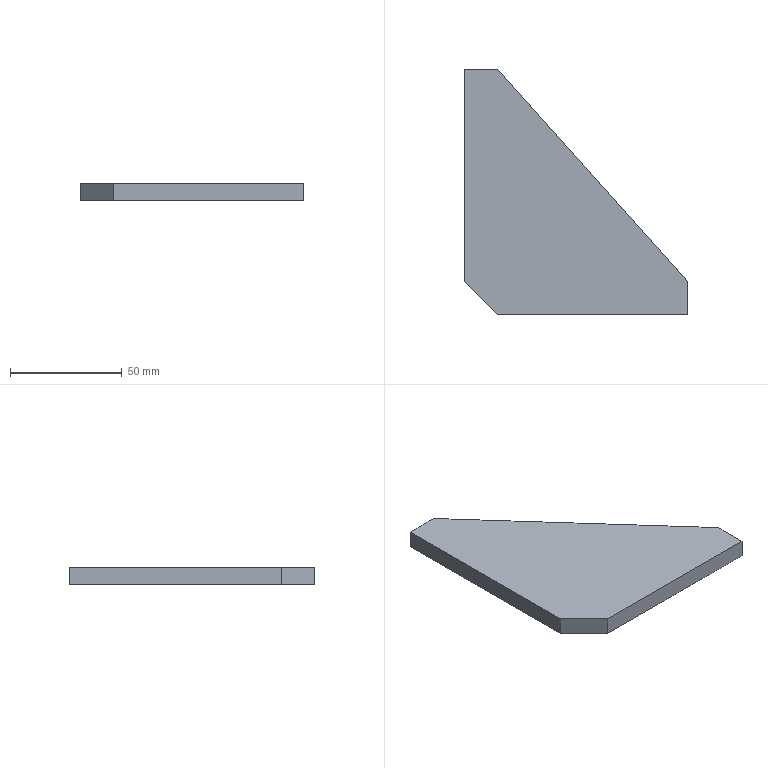Part | SolidWorks | features Chamfer 1, Extrusion 1 | 1 solid | 8 faces | box 100 x 110 x 8 mm | volume 54800 mm3 | plane 8
STEP:
#1=CARTESIAN_POINT('',(0.,110.,0.));
#2=VERTEX_POINT('',#1);
#3=CARTESIAN_POINT('',(0.,15.,0.));
#4=VERTEX_POINT('',#3);
#5=CARTESIAN_POINT('',(0.,110.,0.));
#6=DIRECTION('',(0.,-1.,0.));
#7=VECTOR('',#6,1000.);
#8=LINE('',#5,#7);
#9=EDGE_CURVE('',#2,#4,#8,.T.);
#10=ORIENTED_EDGE('',*,*,#9,.T.);
#11=CARTESIAN_POINT('',(0.,15.,8.));
#12=VERTEX_POINT('',#11);
#13=CARTESIAN_POINT('',(0.,15.,8.));
#14=DIRECTION('',(0.,0.,1.));
#15=VECTOR('',#14,1000.);
#16=LINE('',#13,#15);
#17=EDGE_CURVE('',#4,#12,#16,.T.);
#18=ORIENTED_EDGE('',*,*,#17,.T.);
#19=CARTESIAN_POINT('',(0.,110.,8.));
#20=VERTEX_POINT('',#19);
#21=CARTESIAN_POINT('',(0.,110.,8.));
#22=DIRECTION('',(0.,-1.,0.));
#23=VECTOR('',#22,1000.);
#24=LINE('',#21,#23);
#25=EDGE_CURVE('',#20,#12,#24,.T.);
#26=ORIENTED_EDGE('',*,*,#25,.F.);
#27=CARTESIAN_POINT('',(0.,110.,8.));
#28=DIRECTION('',(0.,0.,-1.));
#29=VECTOR('',#28,1000.);
#30=LINE('',#27,#29);
#31=EDGE_CURVE('',#20,#2,#30,.T.);
#32=ORIENTED_EDGE('',*,*,#31,.T.);
#33=EDGE_LOOP('',(#10,#18,#26,#32));
#34=FACE_OUTER_BOUND('',#33,.T.);
#35=CARTESIAN_POINT('',(0.,110.,8.));
#36=DIRECTION('',(1.,0.,0.));
#37=DIRECTION('',(0.,1.,0.));
#38=AXIS2_PLACEMENT_3D('',#35,#36,#37);
#39=PLANE('',#38);
#40=ADVANCED_FACE('',(#34),#39,.F.);
#41=CARTESIAN_POINT('',(15.,0.,8.));
#42=VERTEX_POINT('',#41);
#43=CARTESIAN_POINT('',(100.,0.,8.));
#44=VERTEX_POINT('',#43);
#45=CARTESIAN_POINT('',(0.,0.,8.));
#46=DIRECTION('',(1.,0.,0.));
#47=VECTOR('',#46,1000.);
#48=LINE('',#45,#47);
#49=EDGE_CURVE('',#42,#44,#48,.T.);
#50=ORIENTED_EDGE('',*,*,#49,.F.);
#51=CARTESIAN_POINT('',(15.,0.,0.));
#52=VERTEX_POINT('',#51);
#53=CARTESIAN_POINT('',(15.,0.,8.));
#54=DIRECTION('',(0.,0.,-1.));
#55=VECTOR('',#54,1000.);
#56=LINE('',#53,#55);
#57=EDGE_CURVE('',#42,#52,#56,.T.);
#58=ORIENTED_EDGE('',*,*,#57,.T.);
#59=CARTESIAN_POINT('',(100.,0.,0.));
#60=VERTEX_POINT('',#59);
#61=CARTESIAN_POINT('',(0.,0.,0.));
#62=DIRECTION('',(1.,0.,0.));
#63=VECTOR('',#62,1000.);
#64=LINE('',#61,#63);
#65=EDGE_CURVE('',#52,#60,#64,.T.);
#66=ORIENTED_EDGE('',*,*,#65,.T.);
#67=CARTESIAN_POINT('',(100.,0.,8.));
#68=DIRECTION('',(0.,0.,-1.));
#69=VECTOR('',#68,1000.);
#70=LINE('',#67,#69);
#71=EDGE_CURVE('',#44,#60,#70,.T.);
#72=ORIENTED_EDGE('',*,*,#71,.F.);
#73=EDGE_LOOP('',(#50,#58,#66,#72));
#74=FACE_OUTER_BOUND('',#73,.T.);
#75=CARTESIAN_POINT('',(0.,0.,8.));
#76=DIRECTION('',(0.,1.,0.));
#77=DIRECTION('',(0.,0.,1.));
#78=AXIS2_PLACEMENT_3D('',#75,#76,#77);
#79=PLANE('',#78);
#80=ADVANCED_FACE('',(#74),#79,.F.);
#81=CARTESIAN_POINT('',(100.,15.,0.));
#82=VERTEX_POINT('',#81);
#83=CARTESIAN_POINT('',(100.,0.,0.));
#84=DIRECTION('',(0.,1.,0.));
#85=VECTOR('',#84,1000.);
#86=LINE('',#83,#85);
#87=EDGE_CURVE('',#60,#82,#86,.T.);
#88=ORIENTED_EDGE('',*,*,#87,.T.);
#89=CARTESIAN_POINT('',(100.,15.,8.));
#90=VERTEX_POINT('',#89);
#91=CARTESIAN_POINT('',(100.,15.,8.));
#92=DIRECTION('',(0.,0.,-1.));
#93=VECTOR('',#92,1000.);
#94=LINE('',#91,#93);
#95=EDGE_CURVE('',#90,#82,#94,.T.);
#96=ORIENTED_EDGE('',*,*,#95,.F.);
#97=CARTESIAN_POINT('',(100.,0.,8.));
#98=DIRECTION('',(0.,1.,0.));
#99=VECTOR('',#98,1000.);
#100=LINE('',#97,#99);
#101=EDGE_CURVE('',#44,#90,#100,.T.);
#102=ORIENTED_EDGE('',*,*,#101,.F.);
#103=ORIENTED_EDGE('',*,*,#71,.T.);
#104=EDGE_LOOP('',(#88,#96,#102,#103));
#105=FACE_OUTER_BOUND('',#104,.T.);
#106=CARTESIAN_POINT('',(100.,0.,8.));
#107=DIRECTION('',(-1.,0.,0.));
#108=DIRECTION('',(0.,0.,1.));
#109=AXIS2_PLACEMENT_3D('',#106,#107,#108);
#110=PLANE('',#109);
#111=ADVANCED_FACE('',(#105),#110,.F.);
#112=CARTESIAN_POINT('',(15.,110.,0.));
#113=VERTEX_POINT('',#112);
#114=CARTESIAN_POINT('',(100.,15.,0.));
#115=DIRECTION('',(-0.6668,0.7452,0.));
#116=VECTOR('',#115,1000.);
#117=LINE('',#114,#116);
#118=EDGE_CURVE('',#82,#113,#117,.T.);
#119=ORIENTED_EDGE('',*,*,#118,.T.);
#120=CARTESIAN_POINT('',(15.,110.,8.));
#121=VERTEX_POINT('',#120);
#122=CARTESIAN_POINT('',(15.,110.,8.));
#123=DIRECTION('',(0.,0.,-1.));
#124=VECTOR('',#123,1000.);
#125=LINE('',#122,#124);
#126=EDGE_CURVE('',#121,#113,#125,.T.);
#127=ORIENTED_EDGE('',*,*,#126,.F.);
#128=CARTESIAN_POINT('',(100.,15.,8.));
#129=DIRECTION('',(-0.6668,0.7452,0.));
#130=VECTOR('',#129,1000.);
#131=LINE('',#128,#130);
#132=EDGE_CURVE('',#90,#121,#131,.T.);
#133=ORIENTED_EDGE('',*,*,#132,.F.);
#134=ORIENTED_EDGE('',*,*,#95,.T.);
#135=EDGE_LOOP('',(#119,#127,#133,#134));
#136=FACE_OUTER_BOUND('',#135,.T.);
#137=CARTESIAN_POINT('',(100.,15.,8.));
#138=DIRECTION('',(-0.7452,-0.6668,0.));
#139=DIRECTION('',(0.6668,-0.7452,0.));
#140=AXIS2_PLACEMENT_3D('',#137,#138,#139);
#141=PLANE('',#140);
#142=ADVANCED_FACE('',(#136),#141,.F.);
#143=CARTESIAN_POINT('',(15.,110.,0.));
#144=DIRECTION('',(-1.,0.,0.));
#145=VECTOR('',#144,1000.);
#146=LINE('',#143,#145);
#147=EDGE_CURVE('',#113,#2,#146,.T.);
#148=ORIENTED_EDGE('',*,*,#147,.T.);
#149=ORIENTED_EDGE('',*,*,#31,.F.);
#150=CARTESIAN_POINT('',(15.,110.,8.));
#151=DIRECTION('',(-1.,0.,0.));
#152=VECTOR('',#151,1000.);
#153=LINE('',#150,#152);
#154=EDGE_CURVE('',#121,#20,#153,.T.);
#155=ORIENTED_EDGE('',*,*,#154,.F.);
#156=ORIENTED_EDGE('',*,*,#126,.T.);
#157=EDGE_LOOP('',(#148,#149,#155,#156));
#158=FACE_OUTER_BOUND('',#157,.T.);
#159=CARTESIAN_POINT('',(15.,110.,8.));
#160=DIRECTION('',(0.,-1.,0.));
#161=DIRECTION('',(0.,0.,-1.));
#162=AXIS2_PLACEMENT_3D('',#159,#160,#161);
#163=PLANE('',#162);
#164=ADVANCED_FACE('',(#158),#163,.F.);
#165=ORIENTED_EDGE('',*,*,#25,.T.);
#166=CARTESIAN_POINT('',(7.5,7.5,8.));
#167=DIRECTION('',(0.7071,-0.7071,0.));
#168=VECTOR('',#167,1000.);
#169=LINE('',#166,#168);
#170=EDGE_CURVE('',#12,#42,#169,.T.);
#171=ORIENTED_EDGE('',*,*,#170,.T.);
#172=ORIENTED_EDGE('',*,*,#49,.T.);
#173=ORIENTED_EDGE('',*,*,#101,.T.);
#174=ORIENTED_EDGE('',*,*,#132,.T.);
#175=ORIENTED_EDGE('',*,*,#154,.T.);
#176=EDGE_LOOP('',(#165,#171,#172,#173,#174,#175));
#177=FACE_OUTER_BOUND('',#176,.T.);
#178=CARTESIAN_POINT('',(0.,0.,8.));
#179=DIRECTION('',(0.,0.,1.));
#180=DIRECTION('',(1.,0.,0.));
#181=AXIS2_PLACEMENT_3D('',#178,#179,#180);
#182=PLANE('',#181);
#183=ADVANCED_FACE('',(#177),#182,.T.);
#184=ORIENTED_EDGE('',*,*,#65,.F.);
#185=CARTESIAN_POINT('',(15.,0.,0.));
#186=DIRECTION('',(-0.7071,0.7071,0.));
#187=VECTOR('',#186,1000.);
#188=LINE('',#185,#187);
#189=EDGE_CURVE('',#52,#4,#188,.T.);
#190=ORIENTED_EDGE('',*,*,#189,.T.);
#191=ORIENTED_EDGE('',*,*,#9,.F.);
#192=ORIENTED_EDGE('',*,*,#147,.F.);
#193=ORIENTED_EDGE('',*,*,#118,.F.);
#194=ORIENTED_EDGE('',*,*,#87,.F.);
#195=EDGE_LOOP('',(#184,#190,#191,#192,#193,#194));
#196=FACE_OUTER_BOUND('',#195,.T.);
#197=CARTESIAN_POINT('',(0.,0.,0.));
#198=DIRECTION('',(0.,0.,1.));
#199=DIRECTION('',(1.,0.,0.));
#200=AXIS2_PLACEMENT_3D('',#197,#198,#199);
#201=PLANE('',#200);
#202=ADVANCED_FACE('',(#196),#201,.F.);
#203=ORIENTED_EDGE('',*,*,#170,.F.);
#204=ORIENTED_EDGE('',*,*,#17,.F.);
#205=ORIENTED_EDGE('',*,*,#189,.F.);
#206=ORIENTED_EDGE('',*,*,#57,.F.);
#207=EDGE_LOOP('',(#203,#204,#205,#206));
#208=FACE_OUTER_BOUND('',#207,.T.);
#209=CARTESIAN_POINT('',(15.,0.,8.));
#210=DIRECTION('',(0.7071,0.7071,0.));
#211=DIRECTION('',(0.,0.,-1.));
#212=AXIS2_PLACEMENT_3D('',#209,#210,#211);
#213=PLANE('',#212);
#214=ADVANCED_FACE('',(#208),#213,.F.);
#215=CLOSED_SHELL('',(#40,#80,#111,#142,#164,#183,#202,#214));
#216=MANIFOLD_SOLID_BREP('',#215);
#217=CARTESIAN_POINT('',(0.,0.,0.));
#218=DIRECTION('',(0.,0.,1.));
#219=DIRECTION('',(1.,0.,0.));
#220=AXIS2_PLACEMENT_3D('',#217,#218,#219);
#221=(LENGTH_UNIT()NAMED_UNIT(*)SI_UNIT(.MILLI.,.METRE.));
#222=UNCERTAINTY_MEASURE_WITH_UNIT(LENGTH_MEASURE(0.00001),#221,'','');
#223=(NAMED_UNIT(*)PLANE_ANGLE_UNIT()SI_UNIT($,.RADIAN.));
#224=(NAMED_UNIT(*)SI_UNIT($,.STERADIAN.)SOLID_ANGLE_UNIT());
#225=(GEOMETRIC_REPRESENTATION_CONTEXT(3)GLOBAL_UNCERTAINTY_ASSIGNED_CONTEXT((#222))GLOBAL_UNIT_ASSIGNED_CONTEXT((#221,#223,#224))REPRESENTATION_CONTEXT('',''));
#226=ADVANCED_BREP_SHAPE_REPRESENTATION('',(#216,#220),#225);